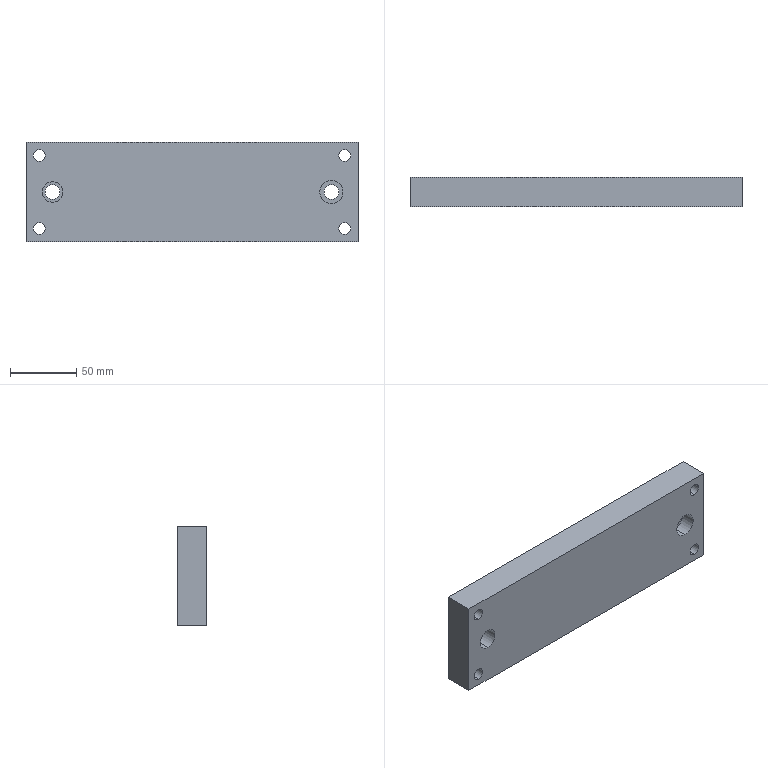Part | STEP file | OP10-031_guide base | 1 solid | 24 faces | box 250 x 22 x 75 mm | volume 400090 mm3 | cylinder 16 | plane 8 | commonest cylinder face diameters 9 x8 11 x4 15.5 x2 17.5 x2